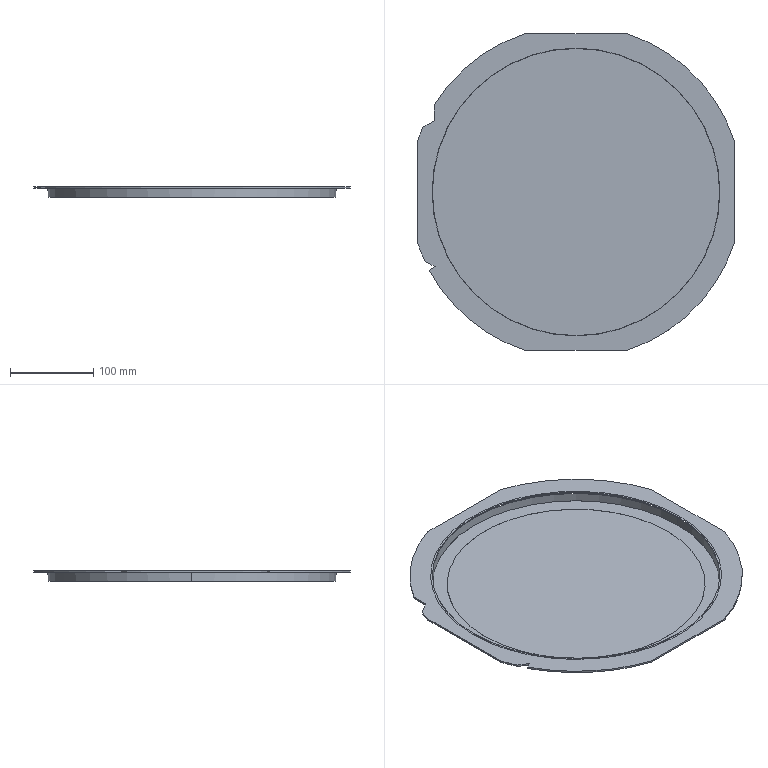Part | NX | features BREP 2 | 2 solids | 31 faces | box 380 x 380 x 12.65 mm | volume 79362 mm3 | plane 15 | cylinder 12 | cone 4 | commonest cylinder face diameters 399.5 x6 310 x2 345.5 x2 349.5 x2
STEP:
#1=CARTESIAN_POINT('',(-172.75,0.,2.));
#2=VERTEX_POINT('',#1);
#3=CARTESIAN_POINT('',(-172.75,0.,1.85));
#4=VERTEX_POINT('',#3);
#5=CARTESIAN_POINT('',(-172.75,0.,1.85));
#6=DIRECTION('',(0.,0.,1.));
#7=VECTOR('',#6,1000.);
#8=LINE('',#5,#7);
#9=EDGE_CURVE('',#2,#4,#8,.F.);
#10=ORIENTED_EDGE('',*,*,#9,.T.);
#11=CARTESIAN_POINT('',(172.75,0.,1.85));
#12=VERTEX_POINT('',#11);
#13=CARTESIAN_POINT('',(0.,0.,1.85));
#14=DIRECTION('',(0.,0.,1.));
#15=DIRECTION('',(1.,0.,0.));
#16=AXIS2_PLACEMENT_3D('',#13,#14,#15);
#17=CIRCLE('',#16,172.75);
#18=EDGE_CURVE('',#12,#4,#17,.T.);
#19=ORIENTED_EDGE('',*,*,#18,.F.);
#20=CARTESIAN_POINT('',(172.75,0.,2.));
#21=VERTEX_POINT('',#20);
#22=CARTESIAN_POINT('',(172.75,0.,1.85));
#23=DIRECTION('',(0.,0.,1.));
#24=VECTOR('',#23,1000.);
#25=LINE('',#22,#24);
#26=EDGE_CURVE('',#21,#12,#25,.F.);
#27=ORIENTED_EDGE('',*,*,#26,.F.);
#28=CARTESIAN_POINT('',(0.,0.,2.));
#29=DIRECTION('',(0.,0.,1.));
#30=DIRECTION('',(1.,0.,0.));
#31=AXIS2_PLACEMENT_3D('',#28,#29,#30);
#32=CIRCLE('',#31,172.75);
#33=EDGE_CURVE('',#21,#2,#32,.T.);
#34=ORIENTED_EDGE('',*,*,#33,.T.);
#35=EDGE_LOOP('',(#10,#19,#27,#34));
#36=FACE_BOUND('',#35,.T.);
#37=CARTESIAN_POINT('',(0.,0.,1.85));
#38=DIRECTION('',(0.,0.,1.));
#39=DIRECTION('',(1.,0.,0.));
#40=AXIS2_PLACEMENT_3D('',#37,#38,#39);
#41=CYLINDRICAL_SURFACE('',#40,172.75);
#42=ADVANCED_FACE('',(#36),#41,.F.);
#43=CARTESIAN_POINT('',(-174.75,0.,1.85));
#44=VERTEX_POINT('',#43);
#45=CARTESIAN_POINT('',(174.75,0.,1.85));
#46=VERTEX_POINT('',#45);
#47=CARTESIAN_POINT('',(0.,0.,1.85));
#48=DIRECTION('',(0.,0.,1.));
#49=DIRECTION('',(1.,0.,0.));
#50=AXIS2_PLACEMENT_3D('',#47,#48,#49);
#51=CIRCLE('',#50,174.75);
#52=EDGE_CURVE('',#44,#46,#51,.T.);
#53=ORIENTED_EDGE('',*,*,#52,.F.);
#54=CARTESIAN_POINT('',(0.,0.,1.85));
#55=DIRECTION('',(0.,0.,1.));
#56=DIRECTION('',(1.,0.,0.));
#57=AXIS2_PLACEMENT_3D('',#54,#55,#56);
#58=CIRCLE('',#57,174.75);
#59=EDGE_CURVE('',#46,#44,#58,.T.);
#60=ORIENTED_EDGE('',*,*,#59,.F.);
#61=EDGE_LOOP('',(#53,#60));
#62=FACE_BOUND('',#61,.T.);
#63=ORIENTED_EDGE('',*,*,#18,.T.);
#64=CARTESIAN_POINT('',(0.,0.,1.85));
#65=DIRECTION('',(0.,0.,1.));
#66=DIRECTION('',(1.,0.,0.));
#67=AXIS2_PLACEMENT_3D('',#64,#65,#66);
#68=CIRCLE('',#67,172.75);
#69=EDGE_CURVE('',#4,#12,#68,.T.);
#70=ORIENTED_EDGE('',*,*,#69,.T.);
#71=EDGE_LOOP('',(#63,#70));
#72=FACE_BOUND('',#71,.T.);
#73=CARTESIAN_POINT('',(0.,0.,1.85));
#74=DIRECTION('',(0.,0.,1.));
#75=DIRECTION('',(1.,0.,0.));
#76=AXIS2_PLACEMENT_3D('',#73,#74,#75);
#77=PLANE('',#76);
#78=ADVANCED_FACE('',(#62,#72),#77,.F.);
#79=CARTESIAN_POINT('',(-169.246,-90.,0.));
#80=VERTEX_POINT('',#79);
#81=CARTESIAN_POINT('',(-176.232,-94.034,0.));
#82=VERTEX_POINT('',#81);
#83=CARTESIAN_POINT('',(-169.246,-90.,0.));
#84=DIRECTION('',(-0.866,-0.5,0.));
#85=VECTOR('',#84,1000.);
#86=LINE('',#83,#85);
#87=EDGE_CURVE('',#80,#82,#86,.T.);
#88=ORIENTED_EDGE('',*,*,#87,.T.);
#89=CARTESIAN_POINT('',(-176.232,-94.034,2.));
#90=VERTEX_POINT('',#89);
#91=CARTESIAN_POINT('',(-176.232,-94.034,2.));
#92=DIRECTION('',(0.,0.,-1.));
#93=VECTOR('',#92,1000.);
#94=LINE('',#91,#93);
#95=EDGE_CURVE('',#90,#82,#94,.T.);
#96=ORIENTED_EDGE('',*,*,#95,.F.);
#97=CARTESIAN_POINT('',(-169.246,-90.,2.));
#98=VERTEX_POINT('',#97);
#99=CARTESIAN_POINT('',(-169.246,-90.,2.));
#100=DIRECTION('',(-0.866,-0.5,0.));
#101=VECTOR('',#100,1000.);
#102=LINE('',#99,#101);
#103=EDGE_CURVE('',#98,#90,#102,.T.);
#104=ORIENTED_EDGE('',*,*,#103,.F.);
#105=CARTESIAN_POINT('',(-169.246,-90.,2.));
#106=DIRECTION('',(0.,0.,-1.));
#107=VECTOR('',#106,1000.);
#108=LINE('',#105,#107);
#109=EDGE_CURVE('',#98,#80,#108,.T.);
#110=ORIENTED_EDGE('',*,*,#109,.T.);
#111=EDGE_LOOP('',(#88,#96,#104,#110));
#112=FACE_BOUND('',#111,.T.);
#113=CARTESIAN_POINT('',(-169.246,-90.,2.));
#114=DIRECTION('',(0.5,-0.866,0.));
#115=DIRECTION('',(0.866,0.5,0.));
#116=AXIS2_PLACEMENT_3D('',#113,#114,#115);
#117=PLANE('',#116);
#118=ADVANCED_FACE('',(#112),#117,.F.);
#119=CARTESIAN_POINT('',(-181.804,-82.75,0.));
#120=VERTEX_POINT('',#119);
#121=CARTESIAN_POINT('',(-169.246,-90.,0.));
#122=DIRECTION('',(0.866,-0.5,0.));
#123=VECTOR('',#122,1000.);
#124=LINE('',#121,#123);
#125=EDGE_CURVE('',#120,#80,#124,.T.);
#126=ORIENTED_EDGE('',*,*,#125,.T.);
#127=ORIENTED_EDGE('',*,*,#109,.F.);
#128=CARTESIAN_POINT('',(-181.804,-82.75,2.));
#129=VERTEX_POINT('',#128);
#130=CARTESIAN_POINT('',(-169.246,-90.,2.));
#131=DIRECTION('',(0.866,-0.5,0.));
#132=VECTOR('',#131,1000.);
#133=LINE('',#130,#132);
#134=EDGE_CURVE('',#129,#98,#133,.T.);
#135=ORIENTED_EDGE('',*,*,#134,.F.);
#136=CARTESIAN_POINT('',(-181.804,-82.75,2.));
#137=DIRECTION('',(0.,0.,-1.));
#138=VECTOR('',#137,1000.);
#139=LINE('',#136,#138);
#140=EDGE_CURVE('',#129,#120,#139,.T.);
#141=ORIENTED_EDGE('',*,*,#140,.T.);
#142=EDGE_LOOP('',(#126,#127,#135,#141));
#143=FACE_BOUND('',#142,.T.);
#144=CARTESIAN_POINT('',(-169.246,-90.,2.));
#145=DIRECTION('',(0.5,0.866,0.));
#146=DIRECTION('',(-0.866,0.5,0.));
#147=AXIS2_PLACEMENT_3D('',#144,#145,#146);
#148=PLANE('',#147);
#149=ADVANCED_FACE('',(#143),#148,.F.);
#150=CARTESIAN_POINT('',(-190.,-61.645,0.));
#151=VERTEX_POINT('',#150);
#152=CARTESIAN_POINT('',(0.,0.,0.));
#153=DIRECTION('',(0.,0.,1.));
#154=DIRECTION('',(1.,0.,0.));
#155=AXIS2_PLACEMENT_3D('',#152,#153,#154);
#156=CIRCLE('',#155,199.75);
#157=EDGE_CURVE('',#151,#120,#156,.T.);
#158=ORIENTED_EDGE('',*,*,#157,.T.);
#159=ORIENTED_EDGE('',*,*,#140,.F.);
#160=CARTESIAN_POINT('',(-190.,-61.645,2.));
#161=VERTEX_POINT('',#160);
#162=CARTESIAN_POINT('',(0.,0.,2.));
#163=DIRECTION('',(0.,0.,1.));
#164=DIRECTION('',(1.,0.,0.));
#165=AXIS2_PLACEMENT_3D('',#162,#163,#164);
#166=CIRCLE('',#165,199.75);
#167=EDGE_CURVE('',#161,#129,#166,.T.);
#168=ORIENTED_EDGE('',*,*,#167,.F.);
#169=CARTESIAN_POINT('',(-190.,-61.645,2.));
#170=DIRECTION('',(0.,0.,-1.));
#171=VECTOR('',#170,1000.);
#172=LINE('',#169,#171);
#173=EDGE_CURVE('',#161,#151,#172,.T.);
#174=ORIENTED_EDGE('',*,*,#173,.T.);
#175=EDGE_LOOP('',(#158,#159,#168,#174));
#176=FACE_BOUND('',#175,.T.);
#177=CARTESIAN_POINT('',(0.,0.,2.));
#178=DIRECTION('',(0.,0.,-1.));
#179=DIRECTION('',(-1.,0.,0.));
#180=AXIS2_PLACEMENT_3D('',#177,#178,#179);
#181=CYLINDRICAL_SURFACE('',#180,199.75);
#182=ADVANCED_FACE('',(#176),#181,.T.);
#183=CARTESIAN_POINT('',(-190.,61.645,0.));
#184=VERTEX_POINT('',#183);
#185=CARTESIAN_POINT('',(-190.,-61.645,0.));
#186=DIRECTION('',(0.,-1.,0.));
#187=VECTOR('',#186,1000.);
#188=LINE('',#185,#187);
#189=EDGE_CURVE('',#184,#151,#188,.T.);
#190=ORIENTED_EDGE('',*,*,#189,.T.);
#191=ORIENTED_EDGE('',*,*,#173,.F.);
#192=CARTESIAN_POINT('',(-190.,61.645,2.));
#193=VERTEX_POINT('',#192);
#194=CARTESIAN_POINT('',(-190.,-61.645,2.));
#195=DIRECTION('',(0.,-1.,0.));
#196=VECTOR('',#195,1000.);
#197=LINE('',#194,#196);
#198=EDGE_CURVE('',#193,#161,#197,.T.);
#199=ORIENTED_EDGE('',*,*,#198,.F.);
#200=CARTESIAN_POINT('',(-190.,61.645,2.));
#201=DIRECTION('',(0.,0.,-1.));
#202=VECTOR('',#201,1000.);
#203=LINE('',#200,#202);
#204=EDGE_CURVE('',#193,#184,#203,.T.);
#205=ORIENTED_EDGE('',*,*,#204,.T.);
#206=EDGE_LOOP('',(#190,#191,#199,#205));
#207=FACE_BOUND('',#206,.T.);
#208=CARTESIAN_POINT('',(-190.,-61.645,2.));
#209=DIRECTION('',(1.,0.,0.));
#210=DIRECTION('',(0.,0.,-1.));
#211=AXIS2_PLACEMENT_3D('',#208,#209,#210);
#212=PLANE('',#211);
#213=ADVANCED_FACE('',(#207),#212,.F.);
#214=CARTESIAN_POINT('',(-184.015,77.709,0.));
#215=VERTEX_POINT('',#214);
#216=CARTESIAN_POINT('',(0.,0.,0.));
#217=DIRECTION('',(0.,0.,1.));
#218=DIRECTION('',(1.,0.,0.));
#219=AXIS2_PLACEMENT_3D('',#216,#217,#218);
#220=CIRCLE('',#219,199.75);
#221=EDGE_CURVE('',#215,#184,#220,.T.);
#222=ORIENTED_EDGE('',*,*,#221,.T.);
#223=ORIENTED_EDGE('',*,*,#204,.F.);
#224=CARTESIAN_POINT('',(-184.015,77.709,2.));
#225=VERTEX_POINT('',#224);
#226=CARTESIAN_POINT('',(0.,0.,2.));
#227=DIRECTION('',(0.,0.,1.));
#228=DIRECTION('',(1.,0.,0.));
#229=AXIS2_PLACEMENT_3D('',#226,#227,#228);
#230=CIRCLE('',#229,199.75);
#231=EDGE_CURVE('',#225,#193,#230,.T.);
#232=ORIENTED_EDGE('',*,*,#231,.F.);
#233=CARTESIAN_POINT('',(-184.015,77.709,2.));
#234=DIRECTION('',(0.,0.,-1.));
#235=VECTOR('',#234,1000.);
#236=LINE('',#233,#235);
#237=EDGE_CURVE('',#225,#215,#236,.T.);
#238=ORIENTED_EDGE('',*,*,#237,.T.);
#239=EDGE_LOOP('',(#222,#223,#232,#238));
#240=FACE_BOUND('',#239,.T.);
#241=CARTESIAN_POINT('',(0.,0.,2.));
#242=DIRECTION('',(0.,0.,-1.));
#243=DIRECTION('',(-1.,0.,0.));
#244=AXIS2_PLACEMENT_3D('',#241,#242,#243);
#245=CYLINDRICAL_SURFACE('',#244,199.75);
#246=ADVANCED_FACE('',(#240),#245,.T.);
#247=CARTESIAN_POINT('',(-170.,85.8,0.));
#248=VERTEX_POINT('',#247);
#249=CARTESIAN_POINT('',(-170.,85.8,0.));
#250=DIRECTION('',(-0.866,-0.5,0.));
#251=VECTOR('',#250,1000.);
#252=LINE('',#249,#251);
#253=EDGE_CURVE('',#248,#215,#252,.T.);
#254=ORIENTED_EDGE('',*,*,#253,.T.);
#255=ORIENTED_EDGE('',*,*,#237,.F.);
#256=CARTESIAN_POINT('',(-170.,85.8,2.));
#257=VERTEX_POINT('',#256);
#258=CARTESIAN_POINT('',(-170.,85.8,2.));
#259=DIRECTION('',(-0.866,-0.5,0.));
#260=VECTOR('',#259,1000.);
#261=LINE('',#258,#260);
#262=EDGE_CURVE('',#257,#225,#261,.T.);
#263=ORIENTED_EDGE('',*,*,#262,.F.);
#264=CARTESIAN_POINT('',(-170.,85.8,2.));
#265=DIRECTION('',(0.,0.,-1.));
#266=VECTOR('',#265,1000.);
#267=LINE('',#264,#266);
#268=EDGE_CURVE('',#257,#248,#267,.T.);
#269=ORIENTED_EDGE('',*,*,#268,.T.);
#270=EDGE_LOOP('',(#254,#255,#263,#269));
#271=FACE_BOUND('',#270,.T.);
#272=CARTESIAN_POINT('',(-170.,85.8,2.));
#273=DIRECTION('',(0.5,-0.866,0.));
#274=DIRECTION('',(0.866,0.5,0.));
#275=AXIS2_PLACEMENT_3D('',#272,#273,#274);
#276=PLANE('',#275);
#277=ADVANCED_FACE('',(#271),#276,.F.);
#278=CARTESIAN_POINT('',(-170.,104.881,0.));
#279=VERTEX_POINT('',#278);
#280=CARTESIAN_POINT('',(-170.,85.8,0.));
#281=DIRECTION('',(0.,-1.,0.));
#282=VECTOR('',#281,1000.);
#283=LINE('',#280,#282);
#284=EDGE_CURVE('',#279,#248,#283,.T.);
#285=ORIENTED_EDGE('',*,*,#284,.T.);
#286=ORIENTED_EDGE('',*,*,#268,.F.);
#287=CARTESIAN_POINT('',(-170.,104.881,2.));
#288=VERTEX_POINT('',#287);
#289=CARTESIAN_POINT('',(-170.,85.8,2.));
#290=DIRECTION('',(0.,-1.,0.));
#291=VECTOR('',#290,1000.);
#292=LINE('',#289,#291);
#293=EDGE_CURVE('',#288,#257,#292,.T.);
#294=ORIENTED_EDGE('',*,*,#293,.F.);
#295=CARTESIAN_POINT('',(-170.,104.881,2.));
#296=DIRECTION('',(0.,0.,-1.));
#297=VECTOR('',#296,1000.);
#298=LINE('',#295,#297);
#299=EDGE_CURVE('',#288,#279,#298,.T.);
#300=ORIENTED_EDGE('',*,*,#299,.T.);
#301=EDGE_LOOP('',(#285,#286,#294,#300));
#302=FACE_BOUND('',#301,.T.);
#303=CARTESIAN_POINT('',(-170.,85.8,2.));
#304=DIRECTION('',(1.,0.,0.));
#305=DIRECTION('',(0.,0.,-1.));
#306=AXIS2_PLACEMENT_3D('',#303,#304,#305);
#307=PLANE('',#306);
#308=ADVANCED_FACE('',(#302),#307,.F.);
#309=CARTESIAN_POINT('',(-61.645,190.,0.));
#310=VERTEX_POINT('',#309);
#311=CARTESIAN_POINT('',(0.,0.,0.));
#312=DIRECTION('',(0.,0.,1.));
#313=DIRECTION('',(1.,0.,0.));
#314=AXIS2_PLACEMENT_3D('',#311,#312,#313);
#315=CIRCLE('',#314,199.75);
#316=EDGE_CURVE('',#310,#279,#315,.T.);
#317=ORIENTED_EDGE('',*,*,#316,.T.);
#318=ORIENTED_EDGE('',*,*,#299,.F.);
#319=CARTESIAN_POINT('',(-61.645,190.,2.));
#320=VERTEX_POINT('',#319);
#321=CARTESIAN_POINT('',(0.,0.,2.));
#322=DIRECTION('',(0.,0.,1.));
#323=DIRECTION('',(1.,0.,0.));
#324=AXIS2_PLACEMENT_3D('',#321,#322,#323);
#325=CIRCLE('',#324,199.75);
#326=EDGE_CURVE('',#320,#288,#325,.T.);
#327=ORIENTED_EDGE('',*,*,#326,.F.);
#328=CARTESIAN_POINT('',(-61.645,190.,2.));
#329=DIRECTION('',(0.,0.,-1.));
#330=VECTOR('',#329,1000.);
#331=LINE('',#328,#330);
#332=EDGE_CURVE('',#320,#310,#331,.T.);
#333=ORIENTED_EDGE('',*,*,#332,.T.);
#334=EDGE_LOOP('',(#317,#318,#327,#333));
#335=FACE_BOUND('',#334,.T.);
#336=CARTESIAN_POINT('',(0.,0.,2.));
#337=DIRECTION('',(0.,0.,-1.));
#338=DIRECTION('',(-1.,0.,0.));
#339=AXIS2_PLACEMENT_3D('',#336,#337,#338);
#340=CYLINDRICAL_SURFACE('',#339,199.75);
#341=ADVANCED_FACE('',(#335),#340,.T.);
#342=CARTESIAN_POINT('',(61.645,190.,0.));
#343=VERTEX_POINT('',#342);
#344=CARTESIAN_POINT('',(-61.645,190.,0.));
#345=DIRECTION('',(-1.,0.,0.));
#346=VECTOR('',#345,1000.);
#347=LINE('',#344,#346);
#348=EDGE_CURVE('',#343,#310,#347,.T.);
#349=ORIENTED_EDGE('',*,*,#348,.T.);
#350=ORIENTED_EDGE('',*,*,#332,.F.);
#351=CARTESIAN_POINT('',(61.645,190.,2.));
#352=VERTEX_POINT('',#351);
#353=CARTESIAN_POINT('',(-61.645,190.,2.));
#354=DIRECTION('',(-1.,0.,0.));
#355=VECTOR('',#354,1000.);
#356=LINE('',#353,#355);
#357=EDGE_CURVE('',#352,#320,#356,.T.);
#358=ORIENTED_EDGE('',*,*,#357,.F.);
#359=CARTESIAN_POINT('',(61.645,190.,2.));
#360=DIRECTION('',(0.,0.,-1.));
#361=VECTOR('',#360,1000.);
#362=LINE('',#359,#361);
#363=EDGE_CURVE('',#352,#343,#362,.T.);
#364=ORIENTED_EDGE('',*,*,#363,.T.);
#365=EDGE_LOOP('',(#349,#350,#358,#364));
#366=FACE_BOUND('',#365,.T.);
#367=CARTESIAN_POINT('',(-61.645,190.,2.));
#368=DIRECTION('',(0.,-1.,0.));
#369=DIRECTION('',(0.,0.,-1.));
#370=AXIS2_PLACEMENT_3D('',#367,#368,#369);
#371=PLANE('',#370);
#372=ADVANCED_FACE('',(#366),#371,.F.);
#373=CARTESIAN_POINT('',(190.,61.645,0.));
#374=VERTEX_POINT('',#373);
#375=CARTESIAN_POINT('',(0.,0.,0.));
#376=DIRECTION('',(0.,0.,1.));
#377=DIRECTION('',(1.,0.,0.));
#378=AXIS2_PLACEMENT_3D('',#375,#376,#377);
#379=CIRCLE('',#378,199.75);
#380=EDGE_CURVE('',#374,#343,#379,.T.);
#381=ORIENTED_EDGE('',*,*,#380,.T.);
#382=ORIENTED_EDGE('',*,*,#363,.F.);
#383=CARTESIAN_POINT('',(190.,61.645,2.));
#384=VERTEX_POINT('',#383);
#385=CARTESIAN_POINT('',(0.,0.,2.));
#386=DIRECTION('',(0.,0.,1.));
#387=DIRECTION('',(1.,0.,0.));
#388=AXIS2_PLACEMENT_3D('',#385,#386,#387);
#389=CIRCLE('',#388,199.75);
#390=EDGE_CURVE('',#384,#352,#389,.T.);
#391=ORIENTED_EDGE('',*,*,#390,.F.);
#392=CARTESIAN_POINT('',(190.,61.645,2.));
#393=DIRECTION('',(0.,0.,-1.));
#394=VECTOR('',#393,1000.);
#395=LINE('',#392,#394);
#396=EDGE_CURVE('',#384,#374,#395,.T.);
#397=ORIENTED_EDGE('',*,*,#396,.T.);
#398=EDGE_LOOP('',(#381,#382,#391,#397));
#399=FACE_BOUND('',#398,.T.);
#400=CARTESIAN_POINT('',(0.,0.,2.));
#401=DIRECTION('',(0.,0.,-1.));
#402=DIRECTION('',(-1.,0.,0.));
#403=AXIS2_PLACEMENT_3D('',#400,#401,#402);
#404=CYLINDRICAL_SURFACE('',#403,199.75);
#405=ADVANCED_FACE('',(#399),#404,.T.);
#406=CARTESIAN_POINT('',(190.,-61.645,0.));
#407=VERTEX_POINT('',#406);
#408=CARTESIAN_POINT('',(190.,-61.645,0.));
#409=DIRECTION('',(0.,1.,0.));
#410=VECTOR('',#409,1000.);
#411=LINE('',#408,#410);
#412=EDGE_CURVE('',#407,#374,#411,.T.);
#413=ORIENTED_EDGE('',*,*,#412,.T.);
#414=ORIENTED_EDGE('',*,*,#396,.F.);
#415=CARTESIAN_POINT('',(190.,-61.645,2.));
#416=VERTEX_POINT('',#415);
#417=CARTESIAN_POINT('',(190.,-61.645,2.));
#418=DIRECTION('',(0.,1.,0.));
#419=VECTOR('',#418,1000.);
#420=LINE('',#417,#419);
#421=EDGE_CURVE('',#416,#384,#420,.T.);
#422=ORIENTED_EDGE('',*,*,#421,.F.);
#423=CARTESIAN_POINT('',(190.,-61.645,2.));
#424=DIRECTION('',(0.,0.,-1.));
#425=VECTOR('',#424,1000.);
#426=LINE('',#423,#425);
#427=EDGE_CURVE('',#416,#407,#426,.T.);
#428=ORIENTED_EDGE('',*,*,#427,.T.);
#429=EDGE_LOOP('',(#413,#414,#422,#428));
#430=FACE_BOUND('',#429,.T.);
#431=CARTESIAN_POINT('',(190.,-61.645,2.));
#432=DIRECTION('',(-1.,0.,0.));
#433=DIRECTION('',(0.,0.,1.));
#434=AXIS2_PLACEMENT_3D('',#431,#432,#433);
#435=PLANE('',#434);
#436=ADVANCED_FACE('',(#430),#435,.F.);
#437=CARTESIAN_POINT('',(61.645,-190.,0.));
#438=VERTEX_POINT('',#437);
#439=CARTESIAN_POINT('',(0.,0.,0.));
#440=DIRECTION('',(0.,0.,1.));
#441=DIRECTION('',(1.,0.,0.));
#442=AXIS2_PLACEMENT_3D('',#439,#440,#441);
#443=CIRCLE('',#442,199.75);
#444=EDGE_CURVE('',#438,#407,#443,.T.);
#445=ORIENTED_EDGE('',*,*,#444,.T.);
#446=ORIENTED_EDGE('',*,*,#427,.F.);
#447=CARTESIAN_POINT('',(61.645,-190.,2.));
#448=VERTEX_POINT('',#447);
#449=CARTESIAN_POINT('',(0.,0.,2.));
#450=DIRECTION('',(0.,0.,1.));
#451=DIRECTION('',(1.,0.,0.));
#452=AXIS2_PLACEMENT_3D('',#449,#450,#451);
#453=CIRCLE('',#452,199.75);
#454=EDGE_CURVE('',#448,#416,#453,.T.);
#455=ORIENTED_EDGE('',*,*,#454,.F.);
#456=CARTESIAN_POINT('',(61.645,-190.,2.));
#457=DIRECTION('',(0.,0.,-1.));
#458=VECTOR('',#457,1000.);
#459=LINE('',#456,#458);
#460=EDGE_CURVE('',#448,#438,#459,.T.);
#461=ORIENTED_EDGE('',*,*,#460,.T.);
#462=EDGE_LOOP('',(#445,#446,#455,#461));
#463=FACE_BOUND('',#462,.T.);
#464=CARTESIAN_POINT('',(0.,0.,2.));
#465=DIRECTION('',(0.,0.,-1.));
#466=DIRECTION('',(-1.,0.,0.));
#467=AXIS2_PLACEMENT_3D('',#464,#465,#466);
#468=CYLINDRICAL_SURFACE('',#467,199.75);
#469=ADVANCED_FACE('',(#463),#468,.T.);
#470=CARTESIAN_POINT('',(-61.645,-190.,0.));
#471=VERTEX_POINT('',#470);
#472=CARTESIAN_POINT('',(-61.645,-190.,0.));
#473=DIRECTION('',(1.,0.,0.));
#474=VECTOR('',#473,1000.);
#475=LINE('',#472,#474);
#476=EDGE_CURVE('',#471,#438,#475,.T.);
#477=ORIENTED_EDGE('',*,*,#476,.T.);
#478=ORIENTED_EDGE('',*,*,#460,.F.);
#479=CARTESIAN_POINT('',(-61.645,-190.,2.));
#480=VERTEX_POINT('',#479);
#481=CARTESIAN_POINT('',(-61.645,-190.,2.));
#482=DIRECTION('',(1.,0.,0.));
#483=VECTOR('',#482,1000.);
#484=LINE('',#481,#483);
#485=EDGE_CURVE('',#480,#448,#484,.T.);
#486=ORIENTED_EDGE('',*,*,#485,.F.);
#487=CARTESIAN_POINT('',(-61.645,-190.,2.));
#488=DIRECTION('',(0.,0.,-1.));
#489=VECTOR('',#488,1000.);
#490=LINE('',#487,#489);
#491=EDGE_CURVE('',#480,#471,#490,.T.);
#492=ORIENTED_EDGE('',*,*,#491,.T.);
#493=EDGE_LOOP('',(#477,#478,#486,#492));
#494=FACE_BOUND('',#493,.T.);
#495=CARTESIAN_POINT('',(-61.645,-190.,2.));
#496=DIRECTION('',(0.,1.,0.));
#497=DIRECTION('',(0.,0.,1.));
#498=AXIS2_PLACEMENT_3D('',#495,#496,#497);
#499=PLANE('',#498);
#500=ADVANCED_FACE('',(#494),#499,.F.);
#501=CARTESIAN_POINT('',(0.,0.,0.));
#502=DIRECTION('',(0.,0.,1.));
#503=DIRECTION('',(1.,0.,0.));
#504=AXIS2_PLACEMENT_3D('',#501,#502,#503);
#505=CIRCLE('',#504,199.75);
#506=EDGE_CURVE('',#82,#471,#505,.T.);
#507=ORIENTED_EDGE('',*,*,#506,.T.);
#508=ORIENTED_EDGE('',*,*,#491,.F.);
#509=CARTESIAN_POINT('',(0.,0.,2.));
#510=DIRECTION('',(0.,0.,1.));
#511=DIRECTION('',(1.,0.,0.));
#512=AXIS2_PLACEMENT_3D('',#509,#510,#511);
#513=CIRCLE('',#512,199.75);
#514=EDGE_CURVE('',#90,#480,#513,.T.);
#515=ORIENTED_EDGE('',*,*,#514,.F.);
#516=ORIENTED_EDGE('',*,*,#95,.T.);
#517=EDGE_LOOP('',(#507,#508,#515,#516));
#518=FACE_BOUND('',#517,.T.);
#519=CARTESIAN_POINT('',(0.,0.,2.));
#520=DIRECTION('',(0.,0.,-1.));
#521=DIRECTION('',(-1.,0.,0.));
#522=AXIS2_PLACEMENT_3D('',#519,#520,#521);
#523=CYLINDRICAL_SURFACE('',#522,199.75);
#524=ADVANCED_FACE('',(#518),#523,.T.);
#525=CARTESIAN_POINT('',(-174.75,0.,0.));
#526=VERTEX_POINT('',#525);
#527=CARTESIAN_POINT('',(174.75,0.,0.));
#528=VERTEX_POINT('',#527);
#529=CARTESIAN_POINT('',(0.,0.,0.));
#530=DIRECTION('',(0.,0.,1.));
#531=DIRECTION('',(1.,0.,0.));
#532=AXIS2_PLACEMENT_3D('',#529,#530,#531);
#533=CIRCLE('',#532,174.75);
#534=EDGE_CURVE('',#526,#528,#533,.T.);
#535=ORIENTED_EDGE('',*,*,#534,.T.);
#536=CARTESIAN_POINT('',(0.,0.,0.));
#537=DIRECTION('',(0.,0.,1.));
#538=DIRECTION('',(1.,0.,0.));
#539=AXIS2_PLACEMENT_3D('',#536,#537,#538);
#540=CIRCLE('',#539,174.75);
#541=EDGE_CURVE('',#528,#526,#540,.T.);
#542=ORIENTED_EDGE('',*,*,#541,.T.);
#543=EDGE_LOOP('',(#535,#542));
#544=FACE_BOUND('',#543,.T.);
#545=ORIENTED_EDGE('',*,*,#506,.F.);
#546=ORIENTED_EDGE('',*,*,#87,.F.);
#547=ORIENTED_EDGE('',*,*,#125,.F.);
#548=ORIENTED_EDGE('',*,*,#157,.F.);
#549=ORIENTED_EDGE('',*,*,#189,.F.);
#550=ORIENTED_EDGE('',*,*,#221,.F.);
#551=ORIENTED_EDGE('',*,*,#253,.F.);
#552=ORIENTED_EDGE('',*,*,#284,.F.);
#553=ORIENTED_EDGE('',*,*,#316,.F.);
#554=ORIENTED_EDGE('',*,*,#348,.F.);
#555=ORIENTED_EDGE('',*,*,#380,.F.);
#556=ORIENTED_EDGE('',*,*,#412,.F.);
#557=ORIENTED_EDGE('',*,*,#444,.F.);
#558=ORIENTED_EDGE('',*,*,#476,.F.);
#559=EDGE_LOOP('',(#545,#546,#547,#548,#549,#550,#551,#552,#553,#554,#555,#556,#557,#558));
#560=FACE_BOUND('',#559,.T.);
#561=CARTESIAN_POINT('',(0.,0.,0.));
#562=DIRECTION('',(0.,0.,1.));
#563=DIRECTION('',(1.,0.,0.));
#564=AXIS2_PLACEMENT_3D('',#561,#562,#563);
#565=PLANE('',#564);
#566=ADVANCED_FACE('',(#544,#560),#565,.F.);
#567=ORIENTED_EDGE('',*,*,#33,.F.);
#568=CARTESIAN_POINT('',(0.,0.,2.));
#569=DIRECTION('',(0.,0.,1.));
#570=DIRECTION('',(1.,0.,0.));
#571=AXIS2_PLACEMENT_3D('',#568,#569,#570);
#572=CIRCLE('',#571,172.75);
#573=EDGE_CURVE('',#2,#21,#572,.T.);
#574=ORIENTED_EDGE('',*,*,#573,.F.);
#575=EDGE_LOOP('',(#567,#574));
#576=FACE_BOUND('',#575,.T.);
#577=ORIENTED_EDGE('',*,*,#514,.T.);
#578=ORIENTED_EDGE('',*,*,#485,.T.);
#579=ORIENTED_EDGE('',*,*,#454,.T.);
#580=ORIENTED_EDGE('',*,*,#421,.T.);
#581=ORIENTED_EDGE('',*,*,#390,.T.);
#582=ORIENTED_EDGE('',*,*,#357,.T.);
#583=ORIENTED_EDGE('',*,*,#326,.T.);
#584=ORIENTED_EDGE('',*,*,#293,.T.);
#585=ORIENTED_EDGE('',*,*,#262,.T.);
#586=ORIENTED_EDGE('',*,*,#231,.T.);
#587=ORIENTED_EDGE('',*,*,#198,.T.);
#588=ORIENTED_EDGE('',*,*,#167,.T.);
#589=ORIENTED_EDGE('',*,*,#134,.T.);
#590=ORIENTED_EDGE('',*,*,#103,.T.);
#591=EDGE_LOOP('',(#577,#578,#579,#580,#581,#582,#583,#584,#585,#586,#587,#588,#589,#590));
#592=FACE_BOUND('',#591,.T.);
#593=CARTESIAN_POINT('',(0.,0.,2.));
#594=DIRECTION('',(0.,0.,1.));
#595=DIRECTION('',(1.,0.,0.));
#596=AXIS2_PLACEMENT_3D('',#593,#594,#595);
#597=PLANE('',#596);
#598=ADVANCED_FACE('',(#576,#592),#597,.T.);
#599=CARTESIAN_POINT('',(174.75,0.,2.));
#600=DIRECTION('',(0.,0.,-1.));
#601=VECTOR('',#600,1000.);
#602=LINE('',#599,#601);
#603=EDGE_CURVE('',#46,#528,#602,.T.);
#604=ORIENTED_EDGE('',*,*,#603,.F.);
#605=ORIENTED_EDGE('',*,*,#59,.T.);
#606=CARTESIAN_POINT('',(-174.75,0.,2.));
#607=DIRECTION('',(0.,0.,-1.));
#608=VECTOR('',#607,1000.);
#609=LINE('',#606,#608);
#610=EDGE_CURVE('',#44,#526,#609,.T.);
#611=ORIENTED_EDGE('',*,*,#610,.T.);
#612=ORIENTED_EDGE('',*,*,#541,.F.);
#613=EDGE_LOOP('',(#604,#605,#611,#612));
#614=FACE_BOUND('',#613,.T.);
#615=CARTESIAN_POINT('',(0.,0.,2.));
#616=DIRECTION('',(0.,0.,-1.));
#617=DIRECTION('',(-1.,0.,0.));
#618=AXIS2_PLACEMENT_3D('',#615,#616,#617);
#619=CYLINDRICAL_SURFACE('',#618,174.75);
#620=ADVANCED_FACE('',(#614),#619,.F.);
#621=ORIENTED_EDGE('',*,*,#52,.T.);
#622=ORIENTED_EDGE('',*,*,#603,.T.);
#623=ORIENTED_EDGE('',*,*,#534,.F.);
#624=ORIENTED_EDGE('',*,*,#610,.F.);
#625=EDGE_LOOP('',(#621,#622,#623,#624));
#626=FACE_BOUND('',#625,.T.);
#627=CARTESIAN_POINT('',(0.,0.,2.));
#628=DIRECTION('',(0.,0.,-1.));
#629=DIRECTION('',(-1.,0.,0.));
#630=AXIS2_PLACEMENT_3D('',#627,#628,#629);
#631=CYLINDRICAL_SURFACE('',#630,174.75);
#632=ADVANCED_FACE('',(#626),#631,.F.);
#633=ORIENTED_EDGE('',*,*,#69,.F.);
#634=ORIENTED_EDGE('',*,*,#9,.F.);
#635=ORIENTED_EDGE('',*,*,#573,.T.);
#636=ORIENTED_EDGE('',*,*,#26,.T.);
#637=EDGE_LOOP('',(#633,#634,#635,#636));
#638=FACE_BOUND('',#637,.T.);
#639=CARTESIAN_POINT('',(0.,0.,1.85));
#640=DIRECTION('',(0.,0.,1.));
#641=DIRECTION('',(1.,0.,0.));
#642=AXIS2_PLACEMENT_3D('',#639,#640,#641);
#643=CYLINDRICAL_SURFACE('',#642,172.75);
#644=ADVANCED_FACE('',(#638),#643,.F.);
#645=CLOSED_SHELL('',(#42,#78,#118,#149,#182,#213,#246,#277,#308,#341,#372,#405,#436,#469,#500,#524,#566,#598,#620,#632,#644));
#646=MANIFOLD_SOLID_BREP('',#645);
#647=CARTESIAN_POINT('',(155.,0.,-10.65));
#648=VERTEX_POINT('',#647);
#649=CARTESIAN_POINT('',(-155.,0.,-10.65));
#650=VERTEX_POINT('',#649);
#651=CARTESIAN_POINT('',(0.,0.,-10.65));
#652=DIRECTION('',(0.,0.,-1.));
#653=DIRECTION('',(-1.,0.,0.));
#654=AXIS2_PLACEMENT_3D('',#651,#652,#653);
#655=CIRCLE('',#654,155.);
#656=EDGE_CURVE('',#648,#650,#655,.T.);
#657=ORIENTED_EDGE('',*,*,#656,.T.);
#658=CARTESIAN_POINT('',(0.,0.,-10.65));
#659=DIRECTION('',(0.,0.,-1.));
#660=DIRECTION('',(-1.,0.,0.));
#661=AXIS2_PLACEMENT_3D('',#658,#659,#660);
#662=CIRCLE('',#661,155.);
#663=EDGE_CURVE('',#650,#648,#662,.T.);
#664=ORIENTED_EDGE('',*,*,#663,.T.);
#665=EDGE_LOOP('',(#657,#664));
#666=FACE_BOUND('',#665,.T.);
#667=CARTESIAN_POINT('',(0.,0.,-10.65));
#668=DIRECTION('',(0.,0.,-1.));
#669=DIRECTION('',(-1.,0.,0.));
#670=AXIS2_PLACEMENT_3D('',#667,#668,#669);
#671=PLANE('',#670);
#672=ADVANCED_FACE('',(#666),#671,.T.);
#673=CARTESIAN_POINT('',(-155.,0.,-10.5));
#674=VERTEX_POINT('',#673);
#675=CARTESIAN_POINT('',(-155.,0.,-10.65));
#676=DIRECTION('',(0.,0.,1.));
#677=VECTOR('',#676,1000.);
#678=LINE('',#675,#677);
#679=EDGE_CURVE('',#674,#650,#678,.F.);
#680=ORIENTED_EDGE('',*,*,#679,.T.);
#681=ORIENTED_EDGE('',*,*,#656,.F.);
#682=CARTESIAN_POINT('',(155.,0.,-10.5));
#683=VERTEX_POINT('',#682);
#684=CARTESIAN_POINT('',(155.,0.,-10.65));
#685=DIRECTION('',(0.,0.,1.));
#686=VECTOR('',#685,1000.);
#687=LINE('',#684,#686);
#688=EDGE_CURVE('',#683,#648,#687,.F.);
#689=ORIENTED_EDGE('',*,*,#688,.F.);
#690=CARTESIAN_POINT('',(0.,0.,-10.5));
#691=DIRECTION('',(0.,0.,-1.));
#692=DIRECTION('',(1.,0.,0.));
#693=AXIS2_PLACEMENT_3D('',#690,#691,#692);
#694=CIRCLE('',#693,155.);
#695=EDGE_CURVE('',#683,#674,#694,.T.);
#696=ORIENTED_EDGE('',*,*,#695,.T.);
#697=EDGE_LOOP('',(#680,#681,#689,#696));
#698=FACE_BOUND('',#697,.T.);
#699=CARTESIAN_POINT('',(0.,0.,-10.65));
#700=DIRECTION('',(0.,0.,1.));
#701=DIRECTION('',(1.,0.,0.));
#702=AXIS2_PLACEMENT_3D('',#699,#700,#701);
#703=CYLINDRICAL_SURFACE('',#702,155.);
#704=ADVANCED_FACE('',(#698),#703,.T.);
#705=CARTESIAN_POINT('',(172.458,0.,-10.35));
#706=VERTEX_POINT('',#705);
#707=CARTESIAN_POINT('',(-172.458,0.,-10.35));
#708=VERTEX_POINT('',#707);
#709=CARTESIAN_POINT('',(0.,0.,-10.35));
#710=DIRECTION('',(0.,0.,1.));
#711=DIRECTION('',(1.,0.,0.));
#712=AXIS2_PLACEMENT_3D('',#709,#710,#711);
#713=CIRCLE('',#712,172.458);
#714=EDGE_CURVE('',#706,#708,#713,.T.);
#715=ORIENTED_EDGE('',*,*,#714,.T.);
#716=CARTESIAN_POINT('',(0.,0.,-10.35));
#717=DIRECTION('',(0.,0.,1.));
#718=DIRECTION('',(1.,0.,0.));
#719=AXIS2_PLACEMENT_3D('',#716,#717,#718);
#720=CIRCLE('',#719,172.458);
#721=EDGE_CURVE('',#708,#706,#720,.T.);
#722=ORIENTED_EDGE('',*,*,#721,.T.);
#723=EDGE_LOOP('',(#715,#722));
#724=FACE_BOUND('',#723,.T.);
#725=CARTESIAN_POINT('',(-172.458,0.,-10.35));
#726=DIRECTION('',(0.,0.,-1.));
#727=DIRECTION('',(-1.,0.,0.));
#728=AXIS2_PLACEMENT_3D('',#725,#726,#727);
#729=PLANE('',#728);
#730=ADVANCED_FACE('',(#724),#729,.F.);
#731=CARTESIAN_POINT('',(-173.,0.,0.));
#732=VERTEX_POINT('',#731);
#733=CARTESIAN_POINT('',(-173.,0.,0.));
#734=DIRECTION('',(-0.05234,0.,0.9986));
#735=VECTOR('',#734,1000.);
#736=LINE('',#733,#735);
#737=EDGE_CURVE('',#732,#708,#736,.F.);
#738=ORIENTED_EDGE('',*,*,#737,.T.);
#739=ORIENTED_EDGE('',*,*,#714,.F.);
#740=CARTESIAN_POINT('',(173.,0.,0.));
#741=VERTEX_POINT('',#740);
#742=CARTESIAN_POINT('',(173.,0.,0.));
#743=DIRECTION('',(0.05234,0.,0.9986));
#744=VECTOR('',#743,1000.);
#745=LINE('',#742,#744);
#746=EDGE_CURVE('',#741,#706,#745,.F.);
#747=ORIENTED_EDGE('',*,*,#746,.F.);
#748=CARTESIAN_POINT('',(0.,0.,0.));
#749=DIRECTION('',(0.,0.,1.));
#750=DIRECTION('',(1.,0.,0.));
#751=AXIS2_PLACEMENT_3D('',#748,#749,#750);
#752=CIRCLE('',#751,173.);
#753=EDGE_CURVE('',#741,#732,#752,.T.);
#754=ORIENTED_EDGE('',*,*,#753,.T.);
#755=EDGE_LOOP('',(#738,#739,#747,#754));
#756=FACE_BOUND('',#755,.T.);
#757=CARTESIAN_POINT('',(0.,0.,0.));
#758=DIRECTION('',(0.,0.,1.));
#759=DIRECTION('',(1.,0.,0.));
#760=AXIS2_PLACEMENT_3D('',#757,#758,#759);
#761=CONICAL_SURFACE('',#760,173.,0.05236);
#762=ADVANCED_FACE('',(#756),#761,.F.);
#763=CARTESIAN_POINT('',(173.15,0.,0.));
#764=VERTEX_POINT('',#763);
#765=CARTESIAN_POINT('',(-173.15,0.,0.));
#766=VERTEX_POINT('',#765);
#767=CARTESIAN_POINT('',(0.,0.,0.));
#768=DIRECTION('',(0.,0.,1.));
#769=DIRECTION('',(1.,0.,0.));
#770=AXIS2_PLACEMENT_3D('',#767,#768,#769);
#771=CIRCLE('',#770,173.15);
#772=EDGE_CURVE('',#764,#766,#771,.T.);
#773=ORIENTED_EDGE('',*,*,#772,.T.);
#774=CARTESIAN_POINT('',(0.,0.,0.));
#775=DIRECTION('',(0.,0.,1.));
#776=DIRECTION('',(1.,0.,0.));
#777=AXIS2_PLACEMENT_3D('',#774,#775,#776);
#778=CIRCLE('',#777,173.15);
#779=EDGE_CURVE('',#766,#764,#778,.T.);
#780=ORIENTED_EDGE('',*,*,#779,.T.);
#781=EDGE_LOOP('',(#773,#780));
#782=FACE_BOUND('',#781,.T.);
#783=ORIENTED_EDGE('',*,*,#753,.F.);
#784=CARTESIAN_POINT('',(0.,0.,0.));
#785=DIRECTION('',(0.,0.,1.));
#786=DIRECTION('',(1.,0.,0.));
#787=AXIS2_PLACEMENT_3D('',#784,#785,#786);
#788=CIRCLE('',#787,173.);
#789=EDGE_CURVE('',#732,#741,#788,.T.);
#790=ORIENTED_EDGE('',*,*,#789,.F.);
#791=EDGE_LOOP('',(#783,#790));
#792=FACE_BOUND('',#791,.T.);
#793=CARTESIAN_POINT('',(-173.15,0.,0.));
#794=DIRECTION('',(0.,0.,-1.));
#795=DIRECTION('',(-1.,0.,0.));
#796=AXIS2_PLACEMENT_3D('',#793,#794,#795);
#797=PLANE('',#796);
#798=ADVANCED_FACE('',(#782,#792),#797,.F.);
#799=CARTESIAN_POINT('',(-172.6,0.,-10.5));
#800=VERTEX_POINT('',#799);
#801=CARTESIAN_POINT('',(-172.6,0.,-10.5));
#802=DIRECTION('',(-0.05234,0.,0.9986));
#803=VECTOR('',#802,1000.);
#804=LINE('',#801,#803);
#805=EDGE_CURVE('',#766,#800,#804,.F.);
#806=ORIENTED_EDGE('',*,*,#805,.T.);
#807=CARTESIAN_POINT('',(172.6,0.,-10.5));
#808=VERTEX_POINT('',#807);
#809=CARTESIAN_POINT('',(0.,0.,-10.5));
#810=DIRECTION('',(0.,0.,1.));
#811=DIRECTION('',(1.,0.,0.));
#812=AXIS2_PLACEMENT_3D('',#809,#810,#811);
#813=CIRCLE('',#812,172.6);
#814=EDGE_CURVE('',#800,#808,#813,.T.);
#815=ORIENTED_EDGE('',*,*,#814,.T.);
#816=CARTESIAN_POINT('',(172.6,0.,-10.5));
#817=DIRECTION('',(0.05234,0.,0.9986));
#818=VECTOR('',#817,1000.);
#819=LINE('',#816,#818);
#820=EDGE_CURVE('',#764,#808,#819,.F.);
#821=ORIENTED_EDGE('',*,*,#820,.F.);
#822=ORIENTED_EDGE('',*,*,#779,.F.);
#823=EDGE_LOOP('',(#806,#815,#821,#822));
#824=FACE_BOUND('',#823,.T.);
#825=CARTESIAN_POINT('',(0.,0.,-10.5));
#826=DIRECTION('',(0.,0.,1.));
#827=DIRECTION('',(1.,0.,0.));
#828=AXIS2_PLACEMENT_3D('',#825,#826,#827);
#829=CONICAL_SURFACE('',#828,172.6,0.05236);
#830=ADVANCED_FACE('',(#824),#829,.T.);
#831=CARTESIAN_POINT('',(0.,0.,-10.5));
#832=DIRECTION('',(0.,0.,1.));
#833=DIRECTION('',(1.,0.,0.));
#834=AXIS2_PLACEMENT_3D('',#831,#832,#833);
#835=CIRCLE('',#834,172.6);
#836=EDGE_CURVE('',#808,#800,#835,.T.);
#837=ORIENTED_EDGE('',*,*,#836,.F.);
#838=ORIENTED_EDGE('',*,*,#814,.F.);
#839=EDGE_LOOP('',(#837,#838));
#840=FACE_BOUND('',#839,.T.);
#841=ORIENTED_EDGE('',*,*,#695,.F.);
#842=CARTESIAN_POINT('',(0.,0.,-10.5));
#843=DIRECTION('',(0.,0.,-1.));
#844=DIRECTION('',(1.,0.,0.));
#845=AXIS2_PLACEMENT_3D('',#842,#843,#844);
#846=CIRCLE('',#845,155.);
#847=EDGE_CURVE('',#674,#683,#846,.T.);
#848=ORIENTED_EDGE('',*,*,#847,.F.);
#849=EDGE_LOOP('',(#841,#848));
#850=FACE_BOUND('',#849,.T.);
#851=CARTESIAN_POINT('',(0.,0.,-10.5));
#852=DIRECTION('',(0.,0.,1.));
#853=DIRECTION('',(1.,0.,0.));
#854=AXIS2_PLACEMENT_3D('',#851,#852,#853);
#855=PLANE('',#854);
#856=ADVANCED_FACE('',(#840,#850),#855,.F.);
#857=ORIENTED_EDGE('',*,*,#836,.T.);
#858=ORIENTED_EDGE('',*,*,#805,.F.);
#859=ORIENTED_EDGE('',*,*,#772,.F.);
#860=ORIENTED_EDGE('',*,*,#820,.T.);
#861=EDGE_LOOP('',(#857,#858,#859,#860));
#862=FACE_BOUND('',#861,.T.);
#863=CARTESIAN_POINT('',(0.,0.,-10.5));
#864=DIRECTION('',(0.,0.,1.));
#865=DIRECTION('',(1.,0.,0.));
#866=AXIS2_PLACEMENT_3D('',#863,#864,#865);
#867=CONICAL_SURFACE('',#866,172.6,0.05236);
#868=ADVANCED_FACE('',(#862),#867,.T.);
#869=ORIENTED_EDGE('',*,*,#721,.F.);
#870=ORIENTED_EDGE('',*,*,#737,.F.);
#871=ORIENTED_EDGE('',*,*,#789,.T.);
#872=ORIENTED_EDGE('',*,*,#746,.T.);
#873=EDGE_LOOP('',(#869,#870,#871,#872));
#874=FACE_BOUND('',#873,.T.);
#875=CARTESIAN_POINT('',(0.,0.,0.));
#876=DIRECTION('',(0.,0.,1.));
#877=DIRECTION('',(1.,0.,0.));
#878=AXIS2_PLACEMENT_3D('',#875,#876,#877);
#879=CONICAL_SURFACE('',#878,173.,0.05236);
#880=ADVANCED_FACE('',(#874),#879,.F.);
#881=ORIENTED_EDGE('',*,*,#663,.F.);
#882=ORIENTED_EDGE('',*,*,#679,.F.);
#883=ORIENTED_EDGE('',*,*,#847,.T.);
#884=ORIENTED_EDGE('',*,*,#688,.T.);
#885=EDGE_LOOP('',(#881,#882,#883,#884));
#886=FACE_BOUND('',#885,.T.);
#887=CARTESIAN_POINT('',(0.,0.,-10.65));
#888=DIRECTION('',(0.,0.,1.));
#889=DIRECTION('',(1.,0.,0.));
#890=AXIS2_PLACEMENT_3D('',#887,#888,#889);
#891=CYLINDRICAL_SURFACE('',#890,155.);
#892=ADVANCED_FACE('',(#886),#891,.T.);
#893=CLOSED_SHELL('',(#672,#704,#730,#762,#798,#830,#856,#868,#880,#892));
#894=MANIFOLD_SOLID_BREP('',#893);
#895=(LENGTH_UNIT()NAMED_UNIT(*)SI_UNIT(.MILLI.,.METRE.));
#896=UNCERTAINTY_MEASURE_WITH_UNIT(LENGTH_MEASURE(0.00001),#895,'','');
#897=(NAMED_UNIT(*)PLANE_ANGLE_UNIT()SI_UNIT($,.RADIAN.));
#898=(NAMED_UNIT(*)SI_UNIT($,.STERADIAN.)SOLID_ANGLE_UNIT());
#899=(GEOMETRIC_REPRESENTATION_CONTEXT(3)GLOBAL_UNCERTAINTY_ASSIGNED_CONTEXT((#896))GLOBAL_UNIT_ASSIGNED_CONTEXT((#895,#897,#898))REPRESENTATION_CONTEXT('',''));
#900=ADVANCED_BREP_SHAPE_REPRESENTATION('',(#646,#894),#899);